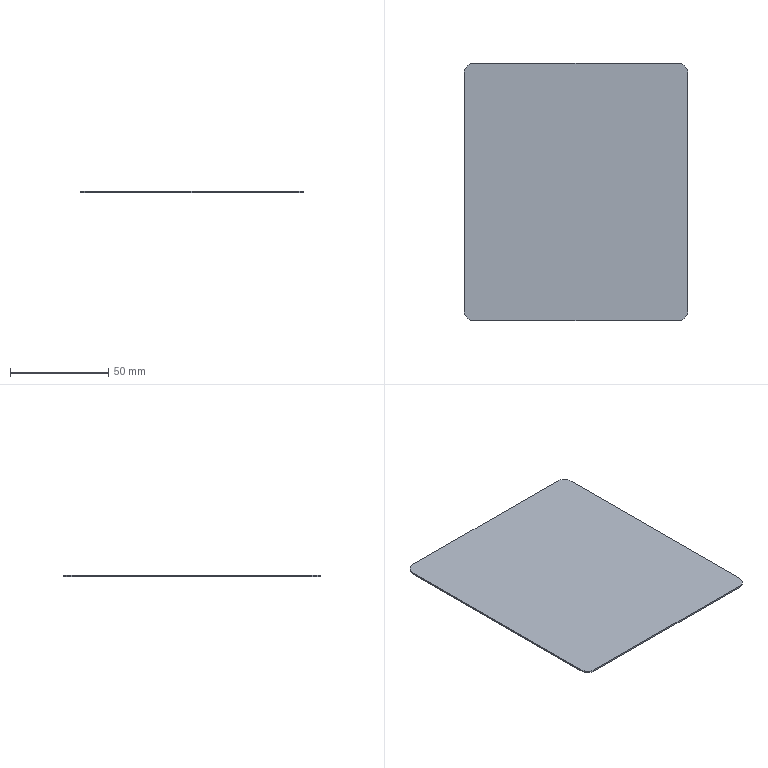Part | STEP file | TY.NE-0002-01-008A Mouse pad-dddeger | 1 solid | 10 faces | box 114 x 131 x 0.8 mm | volume 11930 mm3 | plane 6 | cylinder 4 | commonest cylinder face diameters 10 x4
STEP:
#1=CARTESIAN_POINT('',(0.,0.,0.));
#2=DIRECTION('',(0.,0.,1.));
#3=DIRECTION('',(1.,0.,0.));
#4=AXIS2_PLACEMENT_3D('',#1,#2,#3);
#5=CARTESIAN_POINT('',(57.,-60.5,0.8));
#6=VERTEX_POINT('',#5);
#7=CARTESIAN_POINT('',(57.,60.5,0.8));
#8=VERTEX_POINT('',#7);
#9=CARTESIAN_POINT('',(57.,-65.5,0.8));
#10=DIRECTION('',(0.,1.,0.));
#11=VECTOR('',#10,1.);
#12=LINE('',#9,#11);
#13=CARTESIAN_POINT('',(57.,-65.5,0.8));
#14=DIRECTION('',(-1.,0.,0.));
#15=DIRECTION('',(0.,0.,1.));
#16=AXIS2_PLACEMENT_3D('',#13,#14,#15);
#17=PLANE('',#16);
#18=CARTESIAN_POINT('',(0.,0.));
#19=DIRECTION('',(0.,1.));
#20=VECTOR('',#19,1.);
#21=LINE('',#18,#20);
#22=(GEOMETRIC_REPRESENTATION_CONTEXT(2)PARAMETRIC_REPRESENTATION_CONTEXT()REPRESENTATION_CONTEXT('',''));
#23=DEFINITIONAL_REPRESENTATION('',(#21),#22);
#24=PCURVE('',#17,#23);
#25=CARTESIAN_POINT('',(0.,0.,0.8));
#26=DIRECTION('',(0.,0.,1.));
#27=DIRECTION('',(1.,0.,0.));
#28=AXIS2_PLACEMENT_3D('',#25,#26,#27);
#29=PLANE('',#28);
#30=CARTESIAN_POINT('',(57.,-65.5));
#31=DIRECTION('',(0.,1.));
#32=VECTOR('',#31,1.);
#33=LINE('',#30,#32);
#34=(GEOMETRIC_REPRESENTATION_CONTEXT(2)PARAMETRIC_REPRESENTATION_CONTEXT()REPRESENTATION_CONTEXT('',''));
#35=DEFINITIONAL_REPRESENTATION('',(#33),#34);
#36=PCURVE('',#29,#35);
#37=SURFACE_CURVE('',#12,(#24,#36),.PCURVE_S1.);
#38=EDGE_CURVE('',#6,#8,#37,.T.);
#39=ORIENTED_EDGE('',*,*,#38,.F.);
#40=CARTESIAN_POINT('',(57.,-60.5,0.));
#41=VERTEX_POINT('',#40);
#42=CARTESIAN_POINT('',(57.,-60.5,0.));
#43=DIRECTION('',(0.,0.,-1.));
#44=VECTOR('',#43,1.);
#45=LINE('',#42,#44);
#46=CARTESIAN_POINT('',(-0.8,5.));
#47=DIRECTION('',(-1.,0.));
#48=VECTOR('',#47,1.);
#49=LINE('',#46,#48);
#50=(GEOMETRIC_REPRESENTATION_CONTEXT(2)PARAMETRIC_REPRESENTATION_CONTEXT()REPRESENTATION_CONTEXT('',''));
#51=DEFINITIONAL_REPRESENTATION('',(#49),#50);
#52=PCURVE('',#17,#51);
#53=CARTESIAN_POINT('',(52.,-60.5,0.8));
#54=DIRECTION('',(0.,0.,1.));
#55=DIRECTION('',(1.,0.,0.));
#56=AXIS2_PLACEMENT_3D('',#53,#54,#55);
#57=CYLINDRICAL_SURFACE('',#56,5.);
#58=CARTESIAN_POINT('',(6.283,-0.8));
#59=DIRECTION('',(0.,-1.));
#60=VECTOR('',#59,1.);
#61=LINE('',#58,#60);
#62=(GEOMETRIC_REPRESENTATION_CONTEXT(2)PARAMETRIC_REPRESENTATION_CONTEXT()REPRESENTATION_CONTEXT('',''));
#63=DEFINITIONAL_REPRESENTATION('',(#61),#62);
#64=PCURVE('',#57,#63);
#65=SURFACE_CURVE('',#45,(#52,#64),.PCURVE_S1.);
#66=EDGE_CURVE('',#6,#41,#65,.T.);
#67=ORIENTED_EDGE('',*,*,#66,.T.);
#68=CARTESIAN_POINT('',(57.,60.5,0.));
#69=VERTEX_POINT('',#68);
#70=CARTESIAN_POINT('',(57.,-65.5,0.));
#71=DIRECTION('',(0.,1.,0.));
#72=VECTOR('',#71,1.);
#73=LINE('',#70,#72);
#74=CARTESIAN_POINT('',(-0.8,0.));
#75=DIRECTION('',(0.,1.));
#76=VECTOR('',#75,1.);
#77=LINE('',#74,#76);
#78=(GEOMETRIC_REPRESENTATION_CONTEXT(2)PARAMETRIC_REPRESENTATION_CONTEXT()REPRESENTATION_CONTEXT('',''));
#79=DEFINITIONAL_REPRESENTATION('',(#77),#78);
#80=PCURVE('',#17,#79);
#81=CARTESIAN_POINT('',(0.,0.,0.));
#82=DIRECTION('',(0.,0.,1.));
#83=DIRECTION('',(1.,0.,0.));
#84=AXIS2_PLACEMENT_3D('',#81,#82,#83);
#85=PLANE('',#84);
#86=CARTESIAN_POINT('',(57.,-65.5));
#87=DIRECTION('',(0.,1.));
#88=VECTOR('',#87,1.);
#89=LINE('',#86,#88);
#90=(GEOMETRIC_REPRESENTATION_CONTEXT(2)PARAMETRIC_REPRESENTATION_CONTEXT()REPRESENTATION_CONTEXT('',''));
#91=DEFINITIONAL_REPRESENTATION('',(#89),#90);
#92=PCURVE('',#85,#91);
#93=SURFACE_CURVE('',#73,(#80,#92),.PCURVE_S1.);
#94=EDGE_CURVE('',#41,#69,#93,.T.);
#95=ORIENTED_EDGE('',*,*,#94,.T.);
#96=CARTESIAN_POINT('',(57.,60.5,0.8));
#97=DIRECTION('',(0.,0.,1.));
#98=VECTOR('',#97,1.);
#99=LINE('',#96,#98);
#100=CARTESIAN_POINT('',(0.,126.));
#101=DIRECTION('',(1.,0.));
#102=VECTOR('',#101,1.);
#103=LINE('',#100,#102);
#104=(GEOMETRIC_REPRESENTATION_CONTEXT(2)PARAMETRIC_REPRESENTATION_CONTEXT()REPRESENTATION_CONTEXT('',''));
#105=DEFINITIONAL_REPRESENTATION('',(#103),#104);
#106=PCURVE('',#17,#105);
#107=CARTESIAN_POINT('',(52.,60.5,0.8));
#108=DIRECTION('',(0.,0.,-1.));
#109=DIRECTION('',(-1.,0.,0.));
#110=AXIS2_PLACEMENT_3D('',#107,#108,#109);
#111=CYLINDRICAL_SURFACE('',#110,5.);
#112=CARTESIAN_POINT('',(3.142,0.));
#113=DIRECTION('',(0.,-1.));
#114=VECTOR('',#113,1.);
#115=LINE('',#112,#114);
#116=(GEOMETRIC_REPRESENTATION_CONTEXT(2)PARAMETRIC_REPRESENTATION_CONTEXT()REPRESENTATION_CONTEXT('',''));
#117=DEFINITIONAL_REPRESENTATION('',(#115),#116);
#118=PCURVE('',#111,#117);
#119=SURFACE_CURVE('',#99,(#106,#118),.PCURVE_S1.);
#120=EDGE_CURVE('',#69,#8,#119,.T.);
#121=ORIENTED_EDGE('',*,*,#120,.T.);
#122=EDGE_LOOP('',(#39,#67,#95,#121));
#123=FACE_BOUND('',#122,.T.);
#124=ADVANCED_FACE('',(#123),#17,.F.);
#125=CARTESIAN_POINT('',(52.,65.5,0.8));
#126=VERTEX_POINT('',#125);
#127=CARTESIAN_POINT('',(-52.,65.5,0.8));
#128=VERTEX_POINT('',#127);
#129=CARTESIAN_POINT('',(57.,65.5,0.8));
#130=DIRECTION('',(-1.,0.,0.));
#131=VECTOR('',#130,1.);
#132=LINE('',#129,#131);
#133=CARTESIAN_POINT('',(57.,65.5,0.8));
#134=DIRECTION('',(0.,-1.,0.));
#135=DIRECTION('',(1.,0.,0.));
#136=AXIS2_PLACEMENT_3D('',#133,#134,#135);
#137=PLANE('',#136);
#138=CARTESIAN_POINT('',(0.,0.));
#139=DIRECTION('',(-1.,0.));
#140=VECTOR('',#139,1.);
#141=LINE('',#138,#140);
#142=(GEOMETRIC_REPRESENTATION_CONTEXT(2)PARAMETRIC_REPRESENTATION_CONTEXT()REPRESENTATION_CONTEXT('',''));
#143=DEFINITIONAL_REPRESENTATION('',(#141),#142);
#144=PCURVE('',#137,#143);
#145=CARTESIAN_POINT('',(57.,65.5));
#146=DIRECTION('',(-1.,0.));
#147=VECTOR('',#146,1.);
#148=LINE('',#145,#147);
#149=(GEOMETRIC_REPRESENTATION_CONTEXT(2)PARAMETRIC_REPRESENTATION_CONTEXT()REPRESENTATION_CONTEXT('',''));
#150=DEFINITIONAL_REPRESENTATION('',(#148),#149);
#151=PCURVE('',#29,#150);
#152=SURFACE_CURVE('',#132,(#144,#151),.PCURVE_S1.);
#153=EDGE_CURVE('',#126,#128,#152,.T.);
#154=ORIENTED_EDGE('',*,*,#153,.F.);
#155=CARTESIAN_POINT('',(52.,65.5,0.));
#156=VERTEX_POINT('',#155);
#157=CARTESIAN_POINT('',(52.,65.5,0.8));
#158=DIRECTION('',(0.,0.,-1.));
#159=VECTOR('',#158,1.);
#160=LINE('',#157,#159);
#161=CARTESIAN_POINT('',(-5.,0.));
#162=DIRECTION('',(0.,-1.));
#163=VECTOR('',#162,1.);
#164=LINE('',#161,#163);
#165=(GEOMETRIC_REPRESENTATION_CONTEXT(2)PARAMETRIC_REPRESENTATION_CONTEXT()REPRESENTATION_CONTEXT('',''));
#166=DEFINITIONAL_REPRESENTATION('',(#164),#165);
#167=PCURVE('',#137,#166);
#168=CARTESIAN_POINT('',(1.571,0.));
#169=DIRECTION('',(0.,1.));
#170=VECTOR('',#169,1.);
#171=LINE('',#168,#170);
#172=(GEOMETRIC_REPRESENTATION_CONTEXT(2)PARAMETRIC_REPRESENTATION_CONTEXT()REPRESENTATION_CONTEXT('',''));
#173=DEFINITIONAL_REPRESENTATION('',(#171),#172);
#174=PCURVE('',#111,#173);
#175=SURFACE_CURVE('',#160,(#167,#174),.PCURVE_S1.);
#176=EDGE_CURVE('',#126,#156,#175,.T.);
#177=ORIENTED_EDGE('',*,*,#176,.T.);
#178=CARTESIAN_POINT('',(-52.,65.5,0.));
#179=VERTEX_POINT('',#178);
#180=CARTESIAN_POINT('',(57.,65.5,0.));
#181=DIRECTION('',(-1.,0.,0.));
#182=VECTOR('',#181,1.);
#183=LINE('',#180,#182);
#184=CARTESIAN_POINT('',(0.,-0.8));
#185=DIRECTION('',(-1.,0.));
#186=VECTOR('',#185,1.);
#187=LINE('',#184,#186);
#188=(GEOMETRIC_REPRESENTATION_CONTEXT(2)PARAMETRIC_REPRESENTATION_CONTEXT()REPRESENTATION_CONTEXT('',''));
#189=DEFINITIONAL_REPRESENTATION('',(#187),#188);
#190=PCURVE('',#137,#189);
#191=CARTESIAN_POINT('',(57.,65.5));
#192=DIRECTION('',(-1.,0.));
#193=VECTOR('',#192,1.);
#194=LINE('',#191,#193);
#195=(GEOMETRIC_REPRESENTATION_CONTEXT(2)PARAMETRIC_REPRESENTATION_CONTEXT()REPRESENTATION_CONTEXT('',''));
#196=DEFINITIONAL_REPRESENTATION('',(#194),#195);
#197=PCURVE('',#85,#196);
#198=SURFACE_CURVE('',#183,(#190,#197),.PCURVE_S1.);
#199=EDGE_CURVE('',#156,#179,#198,.T.);
#200=ORIENTED_EDGE('',*,*,#199,.T.);
#201=CARTESIAN_POINT('',(-52.,65.5,0.8));
#202=DIRECTION('',(0.,0.,1.));
#203=VECTOR('',#202,1.);
#204=LINE('',#201,#203);
#205=CARTESIAN_POINT('',(-109.,0.));
#206=DIRECTION('',(0.,1.));
#207=VECTOR('',#206,1.);
#208=LINE('',#205,#207);
#209=(GEOMETRIC_REPRESENTATION_CONTEXT(2)PARAMETRIC_REPRESENTATION_CONTEXT()REPRESENTATION_CONTEXT('',''));
#210=DEFINITIONAL_REPRESENTATION('',(#208),#209);
#211=PCURVE('',#137,#210);
#212=CARTESIAN_POINT('',(-52.,60.5,0.8));
#213=DIRECTION('',(0.,0.,1.));
#214=DIRECTION('',(1.,0.,0.));
#215=AXIS2_PLACEMENT_3D('',#212,#213,#214);
#216=CYLINDRICAL_SURFACE('',#215,5.);
#217=CARTESIAN_POINT('',(1.571,0.));
#218=DIRECTION('',(0.,1.));
#219=VECTOR('',#218,1.);
#220=LINE('',#217,#219);
#221=(GEOMETRIC_REPRESENTATION_CONTEXT(2)PARAMETRIC_REPRESENTATION_CONTEXT()REPRESENTATION_CONTEXT('',''));
#222=DEFINITIONAL_REPRESENTATION('',(#220),#221);
#223=PCURVE('',#216,#222);
#224=SURFACE_CURVE('',#204,(#211,#223),.PCURVE_S1.);
#225=EDGE_CURVE('',#179,#128,#224,.T.);
#226=ORIENTED_EDGE('',*,*,#225,.T.);
#227=EDGE_LOOP('',(#154,#177,#200,#226));
#228=FACE_BOUND('',#227,.T.);
#229=ADVANCED_FACE('',(#228),#137,.F.);
#230=CARTESIAN_POINT('',(-57.,-60.5,0.));
#231=VERTEX_POINT('',#230);
#232=CARTESIAN_POINT('',(-57.,60.5,0.));
#233=VERTEX_POINT('',#232);
#234=CARTESIAN_POINT('',(-57.,-65.5,0.));
#235=DIRECTION('',(0.,1.,0.));
#236=VECTOR('',#235,1.);
#237=LINE('',#234,#236);
#238=CARTESIAN_POINT('',(-57.,-65.5,0.8));
#239=DIRECTION('',(-1.,0.,0.));
#240=DIRECTION('',(0.,0.,1.));
#241=AXIS2_PLACEMENT_3D('',#238,#239,#240);
#242=PLANE('',#241);
#243=CARTESIAN_POINT('',(-0.8,0.));
#244=DIRECTION('',(0.,1.));
#245=VECTOR('',#244,1.);
#246=LINE('',#243,#245);
#247=(GEOMETRIC_REPRESENTATION_CONTEXT(2)PARAMETRIC_REPRESENTATION_CONTEXT()REPRESENTATION_CONTEXT('',''));
#248=DEFINITIONAL_REPRESENTATION('',(#246),#247);
#249=PCURVE('',#242,#248);
#250=CARTESIAN_POINT('',(-57.,-65.5));
#251=DIRECTION('',(0.,1.));
#252=VECTOR('',#251,1.);
#253=LINE('',#250,#252);
#254=(GEOMETRIC_REPRESENTATION_CONTEXT(2)PARAMETRIC_REPRESENTATION_CONTEXT()REPRESENTATION_CONTEXT('',''));
#255=DEFINITIONAL_REPRESENTATION('',(#253),#254);
#256=PCURVE('',#85,#255);
#257=SURFACE_CURVE('',#237,(#249,#256),.PCURVE_S1.);
#258=EDGE_CURVE('',#231,#233,#257,.T.);
#259=ORIENTED_EDGE('',*,*,#258,.F.);
#260=CARTESIAN_POINT('',(-57.,-60.5,0.8));
#261=VERTEX_POINT('',#260);
#262=CARTESIAN_POINT('',(-57.,-60.5,0.8));
#263=DIRECTION('',(0.,0.,1.));
#264=VECTOR('',#263,1.);
#265=LINE('',#262,#264);
#266=CARTESIAN_POINT('',(0.,5.));
#267=DIRECTION('',(1.,0.));
#268=VECTOR('',#267,1.);
#269=LINE('',#266,#268);
#270=(GEOMETRIC_REPRESENTATION_CONTEXT(2)PARAMETRIC_REPRESENTATION_CONTEXT()REPRESENTATION_CONTEXT('',''));
#271=DEFINITIONAL_REPRESENTATION('',(#269),#270);
#272=PCURVE('',#242,#271);
#273=CARTESIAN_POINT('',(-52.,-60.5,0.8));
#274=DIRECTION('',(0.,0.,-1.));
#275=DIRECTION('',(-1.,0.,0.));
#276=AXIS2_PLACEMENT_3D('',#273,#274,#275);
#277=CYLINDRICAL_SURFACE('',#276,5.);
#278=CARTESIAN_POINT('',(6.283,0.));
#279=DIRECTION('',(0.,-1.));
#280=VECTOR('',#279,1.);
#281=LINE('',#278,#280);
#282=(GEOMETRIC_REPRESENTATION_CONTEXT(2)PARAMETRIC_REPRESENTATION_CONTEXT()REPRESENTATION_CONTEXT('',''));
#283=DEFINITIONAL_REPRESENTATION('',(#281),#282);
#284=PCURVE('',#277,#283);
#285=SURFACE_CURVE('',#265,(#272,#284),.PCURVE_S1.);
#286=EDGE_CURVE('',#231,#261,#285,.T.);
#287=ORIENTED_EDGE('',*,*,#286,.T.);
#288=CARTESIAN_POINT('',(-57.,60.5,0.8));
#289=VERTEX_POINT('',#288);
#290=CARTESIAN_POINT('',(-57.,-65.5,0.8));
#291=DIRECTION('',(0.,1.,0.));
#292=VECTOR('',#291,1.);
#293=LINE('',#290,#292);
#294=CARTESIAN_POINT('',(0.,0.));
#295=DIRECTION('',(0.,1.));
#296=VECTOR('',#295,1.);
#297=LINE('',#294,#296);
#298=(GEOMETRIC_REPRESENTATION_CONTEXT(2)PARAMETRIC_REPRESENTATION_CONTEXT()REPRESENTATION_CONTEXT('',''));
#299=DEFINITIONAL_REPRESENTATION('',(#297),#298);
#300=PCURVE('',#242,#299);
#301=CARTESIAN_POINT('',(-57.,-65.5));
#302=DIRECTION('',(0.,1.));
#303=VECTOR('',#302,1.);
#304=LINE('',#301,#303);
#305=(GEOMETRIC_REPRESENTATION_CONTEXT(2)PARAMETRIC_REPRESENTATION_CONTEXT()REPRESENTATION_CONTEXT('',''));
#306=DEFINITIONAL_REPRESENTATION('',(#304),#305);
#307=PCURVE('',#29,#306);
#308=SURFACE_CURVE('',#293,(#300,#307),.PCURVE_S1.);
#309=EDGE_CURVE('',#261,#289,#308,.T.);
#310=ORIENTED_EDGE('',*,*,#309,.T.);
#311=CARTESIAN_POINT('',(-57.,60.5,0.));
#312=DIRECTION('',(0.,0.,-1.));
#313=VECTOR('',#312,1.);
#314=LINE('',#311,#313);
#315=CARTESIAN_POINT('',(-0.8,126.));
#316=DIRECTION('',(-1.,0.));
#317=VECTOR('',#316,1.);
#318=LINE('',#315,#317);
#319=(GEOMETRIC_REPRESENTATION_CONTEXT(2)PARAMETRIC_REPRESENTATION_CONTEXT()REPRESENTATION_CONTEXT('',''));
#320=DEFINITIONAL_REPRESENTATION('',(#318),#319);
#321=PCURVE('',#242,#320);
#322=CARTESIAN_POINT('',(3.142,-0.8));
#323=DIRECTION('',(0.,-1.));
#324=VECTOR('',#323,1.);
#325=LINE('',#322,#324);
#326=(GEOMETRIC_REPRESENTATION_CONTEXT(2)PARAMETRIC_REPRESENTATION_CONTEXT()REPRESENTATION_CONTEXT('',''));
#327=DEFINITIONAL_REPRESENTATION('',(#325),#326);
#328=PCURVE('',#216,#327);
#329=SURFACE_CURVE('',#314,(#321,#328),.PCURVE_S1.);
#330=EDGE_CURVE('',#289,#233,#329,.T.);
#331=ORIENTED_EDGE('',*,*,#330,.T.);
#332=EDGE_LOOP('',(#259,#287,#310,#331));
#333=FACE_BOUND('',#332,.T.);
#334=ADVANCED_FACE('',(#333),#242,.T.);
#335=CARTESIAN_POINT('',(52.,-65.5,0.8));
#336=VERTEX_POINT('',#335);
#337=CARTESIAN_POINT('',(-52.,-65.5,0.8));
#338=VERTEX_POINT('',#337);
#339=CARTESIAN_POINT('',(57.,-65.5,0.8));
#340=DIRECTION('',(-1.,0.,0.));
#341=VECTOR('',#340,1.);
#342=LINE('',#339,#341);
#343=CARTESIAN_POINT('',(57.,-65.5,0.8));
#344=DIRECTION('',(0.,-1.,0.));
#345=DIRECTION('',(1.,0.,0.));
#346=AXIS2_PLACEMENT_3D('',#343,#344,#345);
#347=PLANE('',#346);
#348=CARTESIAN_POINT('',(0.,0.));
#349=DIRECTION('',(-1.,0.));
#350=VECTOR('',#349,1.);
#351=LINE('',#348,#350);
#352=(GEOMETRIC_REPRESENTATION_CONTEXT(2)PARAMETRIC_REPRESENTATION_CONTEXT()REPRESENTATION_CONTEXT('',''));
#353=DEFINITIONAL_REPRESENTATION('',(#351),#352);
#354=PCURVE('',#347,#353);
#355=CARTESIAN_POINT('',(57.,-65.5));
#356=DIRECTION('',(-1.,0.));
#357=VECTOR('',#356,1.);
#358=LINE('',#355,#357);
#359=(GEOMETRIC_REPRESENTATION_CONTEXT(2)PARAMETRIC_REPRESENTATION_CONTEXT()REPRESENTATION_CONTEXT('',''));
#360=DEFINITIONAL_REPRESENTATION('',(#358),#359);
#361=PCURVE('',#29,#360);
#362=SURFACE_CURVE('',#342,(#354,#361),.PCURVE_S1.);
#363=EDGE_CURVE('',#336,#338,#362,.T.);
#364=ORIENTED_EDGE('',*,*,#363,.T.);
#365=CARTESIAN_POINT('',(-52.,-65.5,0.));
#366=VERTEX_POINT('',#365);
#367=CARTESIAN_POINT('',(-52.,-65.5,0.8));
#368=DIRECTION('',(0.,0.,-1.));
#369=VECTOR('',#368,1.);
#370=LINE('',#367,#369);
#371=CARTESIAN_POINT('',(-109.,0.));
#372=DIRECTION('',(0.,-1.));
#373=VECTOR('',#372,1.);
#374=LINE('',#371,#373);
#375=(GEOMETRIC_REPRESENTATION_CONTEXT(2)PARAMETRIC_REPRESENTATION_CONTEXT()REPRESENTATION_CONTEXT('',''));
#376=DEFINITIONAL_REPRESENTATION('',(#374),#375);
#377=PCURVE('',#347,#376);
#378=CARTESIAN_POINT('',(4.712,0.));
#379=DIRECTION('',(0.,1.));
#380=VECTOR('',#379,1.);
#381=LINE('',#378,#380);
#382=(GEOMETRIC_REPRESENTATION_CONTEXT(2)PARAMETRIC_REPRESENTATION_CONTEXT()REPRESENTATION_CONTEXT('',''));
#383=DEFINITIONAL_REPRESENTATION('',(#381),#382);
#384=PCURVE('',#277,#383);
#385=SURFACE_CURVE('',#370,(#377,#384),.PCURVE_S1.);
#386=EDGE_CURVE('',#338,#366,#385,.T.);
#387=ORIENTED_EDGE('',*,*,#386,.T.);
#388=CARTESIAN_POINT('',(52.,-65.5,0.));
#389=VERTEX_POINT('',#388);
#390=CARTESIAN_POINT('',(57.,-65.5,0.));
#391=DIRECTION('',(-1.,0.,0.));
#392=VECTOR('',#391,1.);
#393=LINE('',#390,#392);
#394=CARTESIAN_POINT('',(0.,-0.8));
#395=DIRECTION('',(-1.,0.));
#396=VECTOR('',#395,1.);
#397=LINE('',#394,#396);
#398=(GEOMETRIC_REPRESENTATION_CONTEXT(2)PARAMETRIC_REPRESENTATION_CONTEXT()REPRESENTATION_CONTEXT('',''));
#399=DEFINITIONAL_REPRESENTATION('',(#397),#398);
#400=PCURVE('',#347,#399);
#401=CARTESIAN_POINT('',(57.,-65.5));
#402=DIRECTION('',(-1.,0.));
#403=VECTOR('',#402,1.);
#404=LINE('',#401,#403);
#405=(GEOMETRIC_REPRESENTATION_CONTEXT(2)PARAMETRIC_REPRESENTATION_CONTEXT()REPRESENTATION_CONTEXT('',''));
#406=DEFINITIONAL_REPRESENTATION('',(#404),#405);
#407=PCURVE('',#85,#406);
#408=SURFACE_CURVE('',#393,(#400,#407),.PCURVE_S1.);
#409=EDGE_CURVE('',#389,#366,#408,.T.);
#410=ORIENTED_EDGE('',*,*,#409,.F.);
#411=CARTESIAN_POINT('',(52.,-65.5,0.8));
#412=DIRECTION('',(0.,0.,1.));
#413=VECTOR('',#412,1.);
#414=LINE('',#411,#413);
#415=CARTESIAN_POINT('',(-5.,0.));
#416=DIRECTION('',(0.,1.));
#417=VECTOR('',#416,1.);
#418=LINE('',#415,#417);
#419=(GEOMETRIC_REPRESENTATION_CONTEXT(2)PARAMETRIC_REPRESENTATION_CONTEXT()REPRESENTATION_CONTEXT('',''));
#420=DEFINITIONAL_REPRESENTATION('',(#418),#419);
#421=PCURVE('',#347,#420);
#422=CARTESIAN_POINT('',(4.712,0.));
#423=DIRECTION('',(0.,1.));
#424=VECTOR('',#423,1.);
#425=LINE('',#422,#424);
#426=(GEOMETRIC_REPRESENTATION_CONTEXT(2)PARAMETRIC_REPRESENTATION_CONTEXT()REPRESENTATION_CONTEXT('',''));
#427=DEFINITIONAL_REPRESENTATION('',(#425),#426);
#428=PCURVE('',#57,#427);
#429=SURFACE_CURVE('',#414,(#421,#428),.PCURVE_S1.);
#430=EDGE_CURVE('',#389,#336,#429,.T.);
#431=ORIENTED_EDGE('',*,*,#430,.T.);
#432=EDGE_LOOP('',(#364,#387,#410,#431));
#433=FACE_BOUND('',#432,.T.);
#434=ADVANCED_FACE('',(#433),#347,.T.);
#435=ORIENTED_EDGE('',*,*,#309,.F.);
#436=CARTESIAN_POINT('',(-52.,-60.5,0.8));
#437=DIRECTION('',(0.,0.,1.));
#438=DIRECTION('',(1.,0.,0.));
#439=AXIS2_PLACEMENT_3D('',#436,#437,#438);
#440=CIRCLE('',#439,5.);
#441=CARTESIAN_POINT('',(-52.,-60.5));
#442=DIRECTION('',(1.,0.));
#443=AXIS2_PLACEMENT_2D('',#441,#442);
#444=CIRCLE('',#443,5.);
#445=(GEOMETRIC_REPRESENTATION_CONTEXT(2)PARAMETRIC_REPRESENTATION_CONTEXT()REPRESENTATION_CONTEXT('',''));
#446=DEFINITIONAL_REPRESENTATION('',(#444),#445);
#447=PCURVE('',#29,#446);
#448=CARTESIAN_POINT('',(9.425,0.));
#449=DIRECTION('',(-1.,0.));
#450=VECTOR('',#449,1.);
#451=LINE('',#448,#450);
#452=(GEOMETRIC_REPRESENTATION_CONTEXT(2)PARAMETRIC_REPRESENTATION_CONTEXT()REPRESENTATION_CONTEXT('',''));
#453=DEFINITIONAL_REPRESENTATION('',(#451),#452);
#454=PCURVE('',#277,#453);
#455=SURFACE_CURVE('',#440,(#447,#454),.PCURVE_S1.);
#456=EDGE_CURVE('',#261,#338,#455,.T.);
#457=ORIENTED_EDGE('',*,*,#456,.T.);
#458=ORIENTED_EDGE('',*,*,#363,.F.);
#459=CARTESIAN_POINT('',(52.,-60.5,0.8));
#460=DIRECTION('',(0.,0.,1.));
#461=DIRECTION('',(1.,0.,0.));
#462=AXIS2_PLACEMENT_3D('',#459,#460,#461);
#463=CIRCLE('',#462,5.);
#464=CARTESIAN_POINT('',(52.,-60.5));
#465=DIRECTION('',(1.,0.));
#466=AXIS2_PLACEMENT_2D('',#464,#465);
#467=CIRCLE('',#466,5.);
#468=(GEOMETRIC_REPRESENTATION_CONTEXT(2)PARAMETRIC_REPRESENTATION_CONTEXT()REPRESENTATION_CONTEXT('',''));
#469=DEFINITIONAL_REPRESENTATION('',(#467),#468);
#470=PCURVE('',#29,#469);
#471=CARTESIAN_POINT('',(0.,0.));
#472=DIRECTION('',(1.,0.));
#473=VECTOR('',#472,1.);
#474=LINE('',#471,#473);
#475=(GEOMETRIC_REPRESENTATION_CONTEXT(2)PARAMETRIC_REPRESENTATION_CONTEXT()REPRESENTATION_CONTEXT('',''));
#476=DEFINITIONAL_REPRESENTATION('',(#474),#475);
#477=PCURVE('',#57,#476);
#478=SURFACE_CURVE('',#463,(#470,#477),.PCURVE_S1.);
#479=EDGE_CURVE('',#336,#6,#478,.T.);
#480=ORIENTED_EDGE('',*,*,#479,.T.);
#481=ORIENTED_EDGE('',*,*,#38,.T.);
#482=CARTESIAN_POINT('',(52.,60.5,0.8));
#483=DIRECTION('',(0.,0.,1.));
#484=DIRECTION('',(1.,0.,0.));
#485=AXIS2_PLACEMENT_3D('',#482,#483,#484);
#486=CIRCLE('',#485,5.);
#487=CARTESIAN_POINT('',(52.,60.5));
#488=DIRECTION('',(1.,0.));
#489=AXIS2_PLACEMENT_2D('',#487,#488);
#490=CIRCLE('',#489,5.);
#491=(GEOMETRIC_REPRESENTATION_CONTEXT(2)PARAMETRIC_REPRESENTATION_CONTEXT()REPRESENTATION_CONTEXT('',''));
#492=DEFINITIONAL_REPRESENTATION('',(#490),#491);
#493=PCURVE('',#29,#492);
#494=CARTESIAN_POINT('',(3.142,0.));
#495=DIRECTION('',(-1.,0.));
#496=VECTOR('',#495,1.);
#497=LINE('',#494,#496);
#498=(GEOMETRIC_REPRESENTATION_CONTEXT(2)PARAMETRIC_REPRESENTATION_CONTEXT()REPRESENTATION_CONTEXT('',''));
#499=DEFINITIONAL_REPRESENTATION('',(#497),#498);
#500=PCURVE('',#111,#499);
#501=SURFACE_CURVE('',#486,(#493,#500),.PCURVE_S1.);
#502=EDGE_CURVE('',#8,#126,#501,.T.);
#503=ORIENTED_EDGE('',*,*,#502,.T.);
#504=ORIENTED_EDGE('',*,*,#153,.T.);
#505=CARTESIAN_POINT('',(-52.,60.5,0.8));
#506=DIRECTION('',(0.,0.,1.));
#507=DIRECTION('',(1.,0.,0.));
#508=AXIS2_PLACEMENT_3D('',#505,#506,#507);
#509=CIRCLE('',#508,5.);
#510=CARTESIAN_POINT('',(-52.,60.5));
#511=DIRECTION('',(1.,0.));
#512=AXIS2_PLACEMENT_2D('',#510,#511);
#513=CIRCLE('',#512,5.);
#514=(GEOMETRIC_REPRESENTATION_CONTEXT(2)PARAMETRIC_REPRESENTATION_CONTEXT()REPRESENTATION_CONTEXT('',''));
#515=DEFINITIONAL_REPRESENTATION('',(#513),#514);
#516=PCURVE('',#29,#515);
#517=CARTESIAN_POINT('',(0.,0.));
#518=DIRECTION('',(1.,0.));
#519=VECTOR('',#518,1.);
#520=LINE('',#517,#519);
#521=(GEOMETRIC_REPRESENTATION_CONTEXT(2)PARAMETRIC_REPRESENTATION_CONTEXT()REPRESENTATION_CONTEXT('',''));
#522=DEFINITIONAL_REPRESENTATION('',(#520),#521);
#523=PCURVE('',#216,#522);
#524=SURFACE_CURVE('',#509,(#516,#523),.PCURVE_S1.);
#525=EDGE_CURVE('',#128,#289,#524,.T.);
#526=ORIENTED_EDGE('',*,*,#525,.T.);
#527=EDGE_LOOP('',(#435,#457,#458,#480,#481,#503,#504,#526));
#528=FACE_BOUND('',#527,.T.);
#529=ADVANCED_FACE('',(#528),#29,.T.);
#530=ORIENTED_EDGE('',*,*,#409,.T.);
#531=CARTESIAN_POINT('',(-52.,-60.5,0.));
#532=DIRECTION('',(0.,0.,-1.));
#533=DIRECTION('',(1.,0.,0.));
#534=AXIS2_PLACEMENT_3D('',#531,#532,#533);
#535=CIRCLE('',#534,5.);
#536=CARTESIAN_POINT('',(-47.,-60.5));
#537=CARTESIAN_POINT('',(-47.,-69.16));
#538=CARTESIAN_POINT('',(-54.5,-64.83));
#539=CARTESIAN_POINT('',(-62.,-60.5));
#540=CARTESIAN_POINT('',(-54.5,-56.17));
#541=CARTESIAN_POINT('',(-47.,-51.84));
#542=CARTESIAN_POINT('',(-47.,-60.5));
#543=(BOUNDED_CURVE()B_SPLINE_CURVE(2,(#536,#537,#538,#539,#540,#541,#542),.UNSPECIFIED.,.T.,.F.)B_SPLINE_CURVE_WITH_KNOTS((1,2,2,2,2,1),(-2.094,0.,2.094,4.189,6.283,8.378),.UNSPECIFIED.)CURVE()GEOMETRIC_REPRESENTATION_ITEM()RATIONAL_B_SPLINE_CURVE((1.,0.5,1.,0.5,1.,0.5,1.))REPRESENTATION_ITEM(''));
#544=(GEOMETRIC_REPRESENTATION_CONTEXT(2)PARAMETRIC_REPRESENTATION_CONTEXT()REPRESENTATION_CONTEXT('',''));
#545=DEFINITIONAL_REPRESENTATION('',(#543),#544);
#546=PCURVE('',#85,#545);
#547=CARTESIAN_POINT('',(3.142,0.8));
#548=DIRECTION('',(1.,0.));
#549=VECTOR('',#548,1.);
#550=LINE('',#547,#549);
#551=(GEOMETRIC_REPRESENTATION_CONTEXT(2)PARAMETRIC_REPRESENTATION_CONTEXT()REPRESENTATION_CONTEXT('',''));
#552=DEFINITIONAL_REPRESENTATION('',(#550),#551);
#553=PCURVE('',#277,#552);
#554=SURFACE_CURVE('',#535,(#546,#553),.PCURVE_S1.);
#555=EDGE_CURVE('',#366,#231,#554,.T.);
#556=ORIENTED_EDGE('',*,*,#555,.T.);
#557=ORIENTED_EDGE('',*,*,#258,.T.);
#558=CARTESIAN_POINT('',(-52.,60.5,0.));
#559=DIRECTION('',(0.,0.,-1.));
#560=DIRECTION('',(1.,0.,0.));
#561=AXIS2_PLACEMENT_3D('',#558,#559,#560);
#562=CIRCLE('',#561,5.);
#563=CARTESIAN_POINT('',(-47.,60.5));
#564=CARTESIAN_POINT('',(-47.,51.84));
#565=CARTESIAN_POINT('',(-54.5,56.17));
#566=CARTESIAN_POINT('',(-62.,60.5));
#567=CARTESIAN_POINT('',(-54.5,64.83));
#568=CARTESIAN_POINT('',(-47.,69.16));
#569=CARTESIAN_POINT('',(-47.,60.5));
#570=(BOUNDED_CURVE()B_SPLINE_CURVE(2,(#563,#564,#565,#566,#567,#568,#569),.UNSPECIFIED.,.T.,.F.)B_SPLINE_CURVE_WITH_KNOTS((1,2,2,2,2,1),(-2.094,0.,2.094,4.189,6.283,8.378),.UNSPECIFIED.)CURVE()GEOMETRIC_REPRESENTATION_ITEM()RATIONAL_B_SPLINE_CURVE((1.,0.5,1.,0.5,1.,0.5,1.))REPRESENTATION_ITEM(''));
#571=(GEOMETRIC_REPRESENTATION_CONTEXT(2)PARAMETRIC_REPRESENTATION_CONTEXT()REPRESENTATION_CONTEXT('',''));
#572=DEFINITIONAL_REPRESENTATION('',(#570),#571);
#573=PCURVE('',#85,#572);
#574=CARTESIAN_POINT('',(6.283,-0.8));
#575=DIRECTION('',(-1.,0.));
#576=VECTOR('',#575,1.);
#577=LINE('',#574,#576);
#578=(GEOMETRIC_REPRESENTATION_CONTEXT(2)PARAMETRIC_REPRESENTATION_CONTEXT()REPRESENTATION_CONTEXT('',''));
#579=DEFINITIONAL_REPRESENTATION('',(#577),#578);
#580=PCURVE('',#216,#579);
#581=SURFACE_CURVE('',#562,(#573,#580),.PCURVE_S1.);
#582=EDGE_CURVE('',#233,#179,#581,.T.);
#583=ORIENTED_EDGE('',*,*,#582,.T.);
#584=ORIENTED_EDGE('',*,*,#199,.F.);
#585=CARTESIAN_POINT('',(52.,60.5,0.));
#586=DIRECTION('',(0.,0.,-1.));
#587=DIRECTION('',(1.,0.,0.));
#588=AXIS2_PLACEMENT_3D('',#585,#586,#587);
#589=CIRCLE('',#588,5.);
#590=CARTESIAN_POINT('',(57.,60.5));
#591=CARTESIAN_POINT('',(57.,51.84));
#592=CARTESIAN_POINT('',(49.5,56.17));
#593=CARTESIAN_POINT('',(42.,60.5));
#594=CARTESIAN_POINT('',(49.5,64.83));
#595=CARTESIAN_POINT('',(57.,69.16));
#596=CARTESIAN_POINT('',(57.,60.5));
#597=(BOUNDED_CURVE()B_SPLINE_CURVE(2,(#590,#591,#592,#593,#594,#595,#596),.UNSPECIFIED.,.T.,.F.)B_SPLINE_CURVE_WITH_KNOTS((1,2,2,2,2,1),(-2.094,0.,2.094,4.189,6.283,8.378),.UNSPECIFIED.)CURVE()GEOMETRIC_REPRESENTATION_ITEM()RATIONAL_B_SPLINE_CURVE((1.,0.5,1.,0.5,1.,0.5,1.))REPRESENTATION_ITEM(''));
#598=(GEOMETRIC_REPRESENTATION_CONTEXT(2)PARAMETRIC_REPRESENTATION_CONTEXT()REPRESENTATION_CONTEXT('',''));
#599=DEFINITIONAL_REPRESENTATION('',(#597),#598);
#600=PCURVE('',#85,#599);
#601=CARTESIAN_POINT('',(-3.142,0.8));
#602=DIRECTION('',(1.,0.));
#603=VECTOR('',#602,1.);
#604=LINE('',#601,#603);
#605=(GEOMETRIC_REPRESENTATION_CONTEXT(2)PARAMETRIC_REPRESENTATION_CONTEXT()REPRESENTATION_CONTEXT('',''));
#606=DEFINITIONAL_REPRESENTATION('',(#604),#605);
#607=PCURVE('',#111,#606);
#608=SURFACE_CURVE('',#589,(#600,#607),.PCURVE_S1.);
#609=EDGE_CURVE('',#156,#69,#608,.T.);
#610=ORIENTED_EDGE('',*,*,#609,.T.);
#611=ORIENTED_EDGE('',*,*,#94,.F.);
#612=CARTESIAN_POINT('',(52.,-60.5,0.));
#613=DIRECTION('',(0.,0.,-1.));
#614=DIRECTION('',(1.,0.,0.));
#615=AXIS2_PLACEMENT_3D('',#612,#613,#614);
#616=CIRCLE('',#615,5.);
#617=CARTESIAN_POINT('',(57.,-60.5));
#618=CARTESIAN_POINT('',(57.,-69.16));
#619=CARTESIAN_POINT('',(49.5,-64.83));
#620=CARTESIAN_POINT('',(42.,-60.5));
#621=CARTESIAN_POINT('',(49.5,-56.17));
#622=CARTESIAN_POINT('',(57.,-51.84));
#623=CARTESIAN_POINT('',(57.,-60.5));
#624=(BOUNDED_CURVE()B_SPLINE_CURVE(2,(#617,#618,#619,#620,#621,#622,#623),.UNSPECIFIED.,.T.,.F.)B_SPLINE_CURVE_WITH_KNOTS((1,2,2,2,2,1),(-2.094,0.,2.094,4.189,6.283,8.378),.UNSPECIFIED.)CURVE()GEOMETRIC_REPRESENTATION_ITEM()RATIONAL_B_SPLINE_CURVE((1.,0.5,1.,0.5,1.,0.5,1.))REPRESENTATION_ITEM(''));
#625=(GEOMETRIC_REPRESENTATION_CONTEXT(2)PARAMETRIC_REPRESENTATION_CONTEXT()REPRESENTATION_CONTEXT('',''));
#626=DEFINITIONAL_REPRESENTATION('',(#624),#625);
#627=PCURVE('',#85,#626);
#628=CARTESIAN_POINT('',(6.283,-0.8));
#629=DIRECTION('',(-1.,0.));
#630=VECTOR('',#629,1.);
#631=LINE('',#628,#630);
#632=(GEOMETRIC_REPRESENTATION_CONTEXT(2)PARAMETRIC_REPRESENTATION_CONTEXT()REPRESENTATION_CONTEXT('',''));
#633=DEFINITIONAL_REPRESENTATION('',(#631),#632);
#634=PCURVE('',#57,#633);
#635=SURFACE_CURVE('',#616,(#627,#634),.PCURVE_S1.);
#636=EDGE_CURVE('',#41,#389,#635,.T.);
#637=ORIENTED_EDGE('',*,*,#636,.T.);
#638=EDGE_LOOP('',(#530,#556,#557,#583,#584,#610,#611,#637));
#639=FACE_BOUND('',#638,.T.);
#640=ADVANCED_FACE('',(#639),#85,.F.);
#641=ORIENTED_EDGE('',*,*,#456,.F.);
#642=ORIENTED_EDGE('',*,*,#286,.F.);
#643=ORIENTED_EDGE('',*,*,#555,.F.);
#644=ORIENTED_EDGE('',*,*,#386,.F.);
#645=EDGE_LOOP('',(#641,#642,#643,#644));
#646=FACE_BOUND('',#645,.T.);
#647=ADVANCED_FACE('',(#646),#277,.T.);
#648=ORIENTED_EDGE('',*,*,#479,.F.);
#649=ORIENTED_EDGE('',*,*,#430,.F.);
#650=ORIENTED_EDGE('',*,*,#636,.F.);
#651=ORIENTED_EDGE('',*,*,#66,.F.);
#652=EDGE_LOOP('',(#648,#649,#650,#651));
#653=FACE_BOUND('',#652,.T.);
#654=ADVANCED_FACE('',(#653),#57,.T.);
#655=ORIENTED_EDGE('',*,*,#502,.F.);
#656=ORIENTED_EDGE('',*,*,#120,.F.);
#657=ORIENTED_EDGE('',*,*,#609,.F.);
#658=ORIENTED_EDGE('',*,*,#176,.F.);
#659=EDGE_LOOP('',(#655,#656,#657,#658));
#660=FACE_BOUND('',#659,.T.);
#661=ADVANCED_FACE('',(#660),#111,.T.);
#662=ORIENTED_EDGE('',*,*,#525,.F.);
#663=ORIENTED_EDGE('',*,*,#225,.F.);
#664=ORIENTED_EDGE('',*,*,#582,.F.);
#665=ORIENTED_EDGE('',*,*,#330,.F.);
#666=EDGE_LOOP('',(#662,#663,#664,#665));
#667=FACE_BOUND('',#666,.T.);
#668=ADVANCED_FACE('',(#667),#216,.T.);
#669=CLOSED_SHELL('',(#124,#229,#334,#434,#529,#640,#647,#654,#661,#668));
#670=MANIFOLD_SOLID_BREP('',#669);
#671=(LENGTH_UNIT()NAMED_UNIT(*)SI_UNIT(.MILLI.,.METRE.));
#672=UNCERTAINTY_MEASURE_WITH_UNIT(LENGTH_MEASURE(0.0000001),#671,'','');
#673=(NAMED_UNIT(*)PLANE_ANGLE_UNIT()SI_UNIT($,.RADIAN.));
#674=(NAMED_UNIT(*)SI_UNIT($,.STERADIAN.)SOLID_ANGLE_UNIT());
#675=(GEOMETRIC_REPRESENTATION_CONTEXT(3)GLOBAL_UNCERTAINTY_ASSIGNED_CONTEXT((#672))GLOBAL_UNIT_ASSIGNED_CONTEXT((#671,#673,#674))REPRESENTATION_CONTEXT('',''));
#676=ADVANCED_BREP_SHAPE_REPRESENTATION('',(#4,#670),#675);